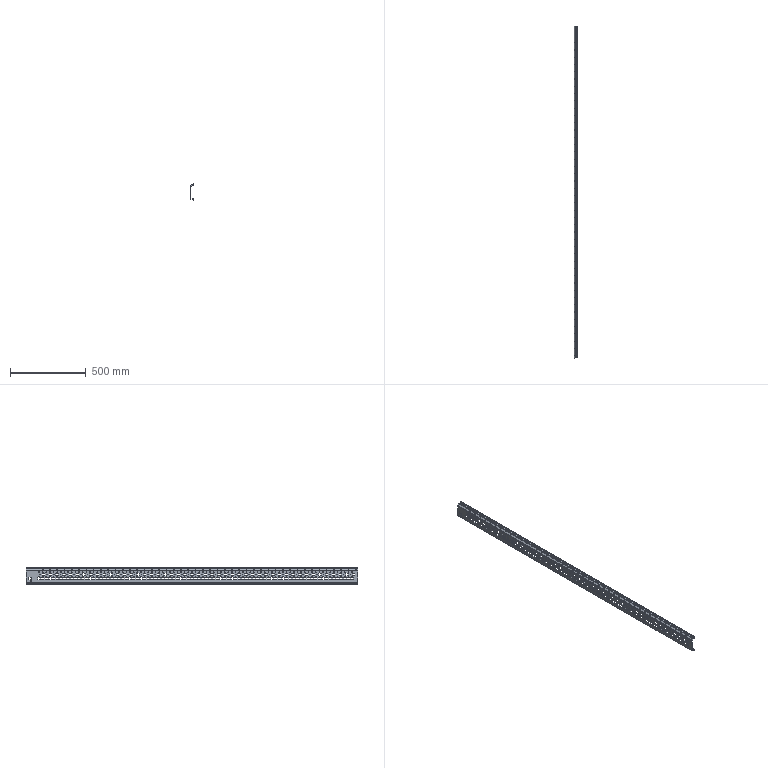Part | NX | features solid 2 | 1 solid | 1694 faces | box 25.68 x 2189 x 114 mm | volume 738720 mm3 | cylinder 1104 | plane 590 | commonest cylinder face diameters 2 x536 4.5 x532 3.2 x28 2.5 x3 7.5 x3 5 x2